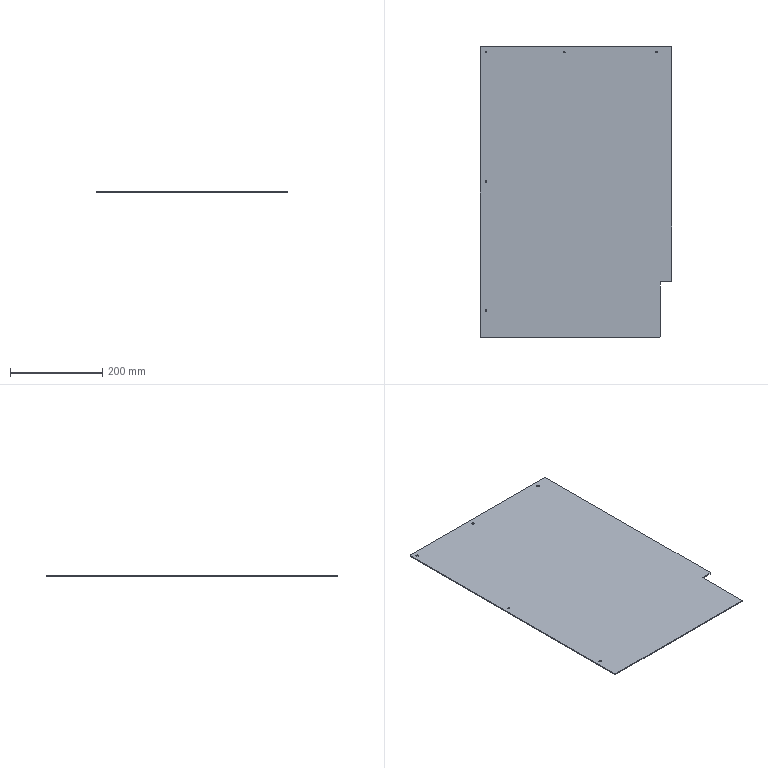Part | STEP file | 11-FG-JX01911 | 1 solid | 34 faces | box 415 x 630 x 2 mm | volume 516605 mm3 | cylinder 16 | cone 10 | plane 8 | commonest cylinder face diameters 3.4 x10 4 x6
STEP:
#1=CARTESIAN_POINT('',(-193.8,-257.,1.66));
#2=VERTEX_POINT('',#1);
#3=CARTESIAN_POINT('',(-197.2,-257.,1.66));
#4=VERTEX_POINT('',#3);
#5=CARTESIAN_POINT('',(-195.5,-257.,1.66));
#6=DIRECTION('',(0.,0.,-1.));
#7=DIRECTION('',(-1.,0.,0.));
#8=AXIS2_PLACEMENT_3D('',#5,#6,#7);
#9=CIRCLE('',#8,1.7);
#10=EDGE_CURVE('',#2,#4,#9,.T.);
#11=ORIENTED_EDGE('',*,*,#10,.F.);
#12=CARTESIAN_POINT('',(-192.14,-257.,0.));
#13=VERTEX_POINT('',#12);
#14=CARTESIAN_POINT('',(-192.14,-257.,0.));
#15=DIRECTION('',(0.7071,0.,-0.7071));
#16=VECTOR('',#15,1000.);
#17=LINE('',#14,#16);
#18=EDGE_CURVE('',#2,#13,#17,.T.);
#19=ORIENTED_EDGE('',*,*,#18,.T.);
#20=CARTESIAN_POINT('',(-198.86,-257.,0.));
#21=VERTEX_POINT('',#20);
#22=CARTESIAN_POINT('',(-195.5,-257.,0.));
#23=DIRECTION('',(0.,0.,-1.));
#24=DIRECTION('',(-1.,0.,0.));
#25=AXIS2_PLACEMENT_3D('',#22,#23,#24);
#26=CIRCLE('',#25,3.36);
#27=EDGE_CURVE('',#13,#21,#26,.T.);
#28=ORIENTED_EDGE('',*,*,#27,.T.);
#29=CARTESIAN_POINT('',(-198.86,-257.,0.));
#30=DIRECTION('',(-0.7071,0.,-0.7071));
#31=VECTOR('',#30,1000.);
#32=LINE('',#29,#31);
#33=EDGE_CURVE('',#4,#21,#32,.T.);
#34=ORIENTED_EDGE('',*,*,#33,.F.);
#35=EDGE_LOOP('',(#11,#19,#28,#34));
#36=FACE_OUTER_BOUND('',#35,.T.);
#37=CARTESIAN_POINT('',(-195.5,-257.,0.));
#38=DIRECTION('',(0.,0.,-1.));
#39=DIRECTION('',(-1.,0.,0.));
#40=AXIS2_PLACEMENT_3D('',#37,#38,#39);
#41=CONICAL_SURFACE('',#40,3.36,0.7854);
#42=ADVANCED_FACE('',(#36),#41,.F.);
#43=CARTESIAN_POINT('',(-193.8,-257.,2.));
#44=VERTEX_POINT('',#43);
#45=CARTESIAN_POINT('',(-197.2,-257.,2.));
#46=VERTEX_POINT('',#45);
#47=CARTESIAN_POINT('',(-195.5,-257.,2.));
#48=DIRECTION('',(0.,0.,-1.));
#49=DIRECTION('',(-1.,0.,0.));
#50=AXIS2_PLACEMENT_3D('',#47,#48,#49);
#51=CIRCLE('',#50,1.7);
#52=EDGE_CURVE('',#44,#46,#51,.T.);
#53=ORIENTED_EDGE('',*,*,#52,.F.);
#54=CARTESIAN_POINT('',(-193.8,-257.,0.));
#55=DIRECTION('',(0.,0.,-1.));
#56=VECTOR('',#55,1000.);
#57=LINE('',#54,#56);
#58=EDGE_CURVE('',#44,#2,#57,.T.);
#59=ORIENTED_EDGE('',*,*,#58,.T.);
#60=ORIENTED_EDGE('',*,*,#10,.T.);
#61=CARTESIAN_POINT('',(-197.2,-257.,0.));
#62=DIRECTION('',(0.,0.,-1.));
#63=VECTOR('',#62,1000.);
#64=LINE('',#61,#63);
#65=EDGE_CURVE('',#46,#4,#64,.T.);
#66=ORIENTED_EDGE('',*,*,#65,.F.);
#67=EDGE_LOOP('',(#53,#59,#60,#66));
#68=FACE_OUTER_BOUND('',#67,.T.);
#69=CARTESIAN_POINT('',(-195.5,-257.,0.));
#70=DIRECTION('',(0.,0.,-1.));
#71=DIRECTION('',(-1.,0.,0.));
#72=AXIS2_PLACEMENT_3D('',#69,#70,#71);
#73=CYLINDRICAL_SURFACE('',#72,1.7);
#74=ADVANCED_FACE('',(#68),#73,.F.);
#75=CARTESIAN_POINT('',(-193.8,23.,1.66));
#76=VERTEX_POINT('',#75);
#77=CARTESIAN_POINT('',(-197.2,23.,1.66));
#78=VERTEX_POINT('',#77);
#79=CARTESIAN_POINT('',(-195.5,23.,1.66));
#80=DIRECTION('',(0.,0.,-1.));
#81=DIRECTION('',(-1.,0.,0.));
#82=AXIS2_PLACEMENT_3D('',#79,#80,#81);
#83=CIRCLE('',#82,1.7);
#84=EDGE_CURVE('',#76,#78,#83,.T.);
#85=ORIENTED_EDGE('',*,*,#84,.F.);
#86=CARTESIAN_POINT('',(-192.14,23.,0.));
#87=VERTEX_POINT('',#86);
#88=CARTESIAN_POINT('',(-192.14,23.,0.));
#89=DIRECTION('',(0.7071,0.,-0.7071));
#90=VECTOR('',#89,1000.);
#91=LINE('',#88,#90);
#92=EDGE_CURVE('',#76,#87,#91,.T.);
#93=ORIENTED_EDGE('',*,*,#92,.T.);
#94=CARTESIAN_POINT('',(-198.86,23.,0.));
#95=VERTEX_POINT('',#94);
#96=CARTESIAN_POINT('',(-195.5,23.,0.));
#97=DIRECTION('',(0.,0.,-1.));
#98=DIRECTION('',(-1.,0.,0.));
#99=AXIS2_PLACEMENT_3D('',#96,#97,#98);
#100=CIRCLE('',#99,3.36);
#101=EDGE_CURVE('',#87,#95,#100,.T.);
#102=ORIENTED_EDGE('',*,*,#101,.T.);
#103=CARTESIAN_POINT('',(-198.86,23.,0.));
#104=DIRECTION('',(-0.7071,0.,-0.7071));
#105=VECTOR('',#104,1000.);
#106=LINE('',#103,#105);
#107=EDGE_CURVE('',#78,#95,#106,.T.);
#108=ORIENTED_EDGE('',*,*,#107,.F.);
#109=EDGE_LOOP('',(#85,#93,#102,#108));
#110=FACE_OUTER_BOUND('',#109,.T.);
#111=CARTESIAN_POINT('',(-195.5,23.,0.));
#112=DIRECTION('',(0.,0.,-1.));
#113=DIRECTION('',(-1.,0.,0.));
#114=AXIS2_PLACEMENT_3D('',#111,#112,#113);
#115=CONICAL_SURFACE('',#114,3.36,0.7854);
#116=ADVANCED_FACE('',(#110),#115,.F.);
#117=CARTESIAN_POINT('',(-193.8,23.,2.));
#118=VERTEX_POINT('',#117);
#119=CARTESIAN_POINT('',(-197.2,23.,2.));
#120=VERTEX_POINT('',#119);
#121=CARTESIAN_POINT('',(-195.5,23.,2.));
#122=DIRECTION('',(0.,0.,-1.));
#123=DIRECTION('',(-1.,0.,0.));
#124=AXIS2_PLACEMENT_3D('',#121,#122,#123);
#125=CIRCLE('',#124,1.7);
#126=EDGE_CURVE('',#118,#120,#125,.T.);
#127=ORIENTED_EDGE('',*,*,#126,.F.);
#128=CARTESIAN_POINT('',(-193.8,23.,0.));
#129=DIRECTION('',(0.,0.,-1.));
#130=VECTOR('',#129,1000.);
#131=LINE('',#128,#130);
#132=EDGE_CURVE('',#118,#76,#131,.T.);
#133=ORIENTED_EDGE('',*,*,#132,.T.);
#134=ORIENTED_EDGE('',*,*,#84,.T.);
#135=CARTESIAN_POINT('',(-197.2,23.,0.));
#136=DIRECTION('',(0.,0.,-1.));
#137=VECTOR('',#136,1000.);
#138=LINE('',#135,#137);
#139=EDGE_CURVE('',#120,#78,#138,.T.);
#140=ORIENTED_EDGE('',*,*,#139,.F.);
#141=EDGE_LOOP('',(#127,#133,#134,#140));
#142=FACE_OUTER_BOUND('',#141,.T.);
#143=CARTESIAN_POINT('',(-195.5,23.,0.));
#144=DIRECTION('',(0.,0.,-1.));
#145=DIRECTION('',(-1.,0.,0.));
#146=AXIS2_PLACEMENT_3D('',#143,#144,#145);
#147=CYLINDRICAL_SURFACE('',#146,1.7);
#148=ADVANCED_FACE('',(#142),#147,.F.);
#149=CARTESIAN_POINT('',(-193.8,303.,1.66));
#150=VERTEX_POINT('',#149);
#151=CARTESIAN_POINT('',(-197.2,303.,1.66));
#152=VERTEX_POINT('',#151);
#153=CARTESIAN_POINT('',(-195.5,303.,1.66));
#154=DIRECTION('',(0.,0.,-1.));
#155=DIRECTION('',(-1.,0.,0.));
#156=AXIS2_PLACEMENT_3D('',#153,#154,#155);
#157=CIRCLE('',#156,1.7);
#158=EDGE_CURVE('',#150,#152,#157,.T.);
#159=ORIENTED_EDGE('',*,*,#158,.F.);
#160=CARTESIAN_POINT('',(-192.14,303.,0.));
#161=VERTEX_POINT('',#160);
#162=CARTESIAN_POINT('',(-192.14,303.,0.));
#163=DIRECTION('',(0.7071,0.,-0.7071));
#164=VECTOR('',#163,1000.);
#165=LINE('',#162,#164);
#166=EDGE_CURVE('',#150,#161,#165,.T.);
#167=ORIENTED_EDGE('',*,*,#166,.T.);
#168=CARTESIAN_POINT('',(-198.86,303.,0.));
#169=VERTEX_POINT('',#168);
#170=CARTESIAN_POINT('',(-195.5,303.,0.));
#171=DIRECTION('',(0.,0.,-1.));
#172=DIRECTION('',(-1.,0.,0.));
#173=AXIS2_PLACEMENT_3D('',#170,#171,#172);
#174=CIRCLE('',#173,3.36);
#175=EDGE_CURVE('',#161,#169,#174,.T.);
#176=ORIENTED_EDGE('',*,*,#175,.T.);
#177=CARTESIAN_POINT('',(-198.86,303.,0.));
#178=DIRECTION('',(-0.7071,0.,-0.7071));
#179=VECTOR('',#178,1000.);
#180=LINE('',#177,#179);
#181=EDGE_CURVE('',#152,#169,#180,.T.);
#182=ORIENTED_EDGE('',*,*,#181,.F.);
#183=EDGE_LOOP('',(#159,#167,#176,#182));
#184=FACE_OUTER_BOUND('',#183,.T.);
#185=CARTESIAN_POINT('',(-195.5,303.,0.));
#186=DIRECTION('',(0.,0.,-1.));
#187=DIRECTION('',(-1.,0.,0.));
#188=AXIS2_PLACEMENT_3D('',#185,#186,#187);
#189=CONICAL_SURFACE('',#188,3.36,0.7854);
#190=ADVANCED_FACE('',(#184),#189,.F.);
#191=CARTESIAN_POINT('',(-193.8,303.,2.));
#192=VERTEX_POINT('',#191);
#193=CARTESIAN_POINT('',(-197.2,303.,2.));
#194=VERTEX_POINT('',#193);
#195=CARTESIAN_POINT('',(-195.5,303.,2.));
#196=DIRECTION('',(0.,0.,-1.));
#197=DIRECTION('',(-1.,0.,0.));
#198=AXIS2_PLACEMENT_3D('',#195,#196,#197);
#199=CIRCLE('',#198,1.7);
#200=EDGE_CURVE('',#192,#194,#199,.T.);
#201=ORIENTED_EDGE('',*,*,#200,.F.);
#202=CARTESIAN_POINT('',(-193.8,303.,0.));
#203=DIRECTION('',(0.,0.,-1.));
#204=VECTOR('',#203,1000.);
#205=LINE('',#202,#204);
#206=EDGE_CURVE('',#192,#150,#205,.T.);
#207=ORIENTED_EDGE('',*,*,#206,.T.);
#208=ORIENTED_EDGE('',*,*,#158,.T.);
#209=CARTESIAN_POINT('',(-197.2,303.,0.));
#210=DIRECTION('',(0.,0.,-1.));
#211=VECTOR('',#210,1000.);
#212=LINE('',#209,#211);
#213=EDGE_CURVE('',#194,#152,#212,.T.);
#214=ORIENTED_EDGE('',*,*,#213,.F.);
#215=EDGE_LOOP('',(#201,#207,#208,#214));
#216=FACE_OUTER_BOUND('',#215,.T.);
#217=CARTESIAN_POINT('',(-195.5,303.,0.));
#218=DIRECTION('',(0.,0.,-1.));
#219=DIRECTION('',(-1.,0.,0.));
#220=AXIS2_PLACEMENT_3D('',#217,#218,#219);
#221=CYLINDRICAL_SURFACE('',#220,1.7);
#222=ADVANCED_FACE('',(#216),#221,.F.);
#223=CARTESIAN_POINT('',(-23.8,303.,1.66));
#224=VERTEX_POINT('',#223);
#225=CARTESIAN_POINT('',(-27.2,303.,1.66));
#226=VERTEX_POINT('',#225);
#227=CARTESIAN_POINT('',(-25.5,303.,1.66));
#228=DIRECTION('',(0.,0.,-1.));
#229=DIRECTION('',(-1.,0.,0.));
#230=AXIS2_PLACEMENT_3D('',#227,#228,#229);
#231=CIRCLE('',#230,1.7);
#232=EDGE_CURVE('',#224,#226,#231,.T.);
#233=ORIENTED_EDGE('',*,*,#232,.F.);
#234=CARTESIAN_POINT('',(-22.14,303.,0.));
#235=VERTEX_POINT('',#234);
#236=CARTESIAN_POINT('',(-22.14,303.,0.));
#237=DIRECTION('',(0.7071,0.,-0.7071));
#238=VECTOR('',#237,1000.);
#239=LINE('',#236,#238);
#240=EDGE_CURVE('',#224,#235,#239,.T.);
#241=ORIENTED_EDGE('',*,*,#240,.T.);
#242=CARTESIAN_POINT('',(-28.86,303.,0.));
#243=VERTEX_POINT('',#242);
#244=CARTESIAN_POINT('',(-25.5,303.,0.));
#245=DIRECTION('',(0.,0.,-1.));
#246=DIRECTION('',(-1.,0.,0.));
#247=AXIS2_PLACEMENT_3D('',#244,#245,#246);
#248=CIRCLE('',#247,3.36);
#249=EDGE_CURVE('',#235,#243,#248,.T.);
#250=ORIENTED_EDGE('',*,*,#249,.T.);
#251=CARTESIAN_POINT('',(-28.86,303.,0.));
#252=DIRECTION('',(-0.7071,0.,-0.7071));
#253=VECTOR('',#252,1000.);
#254=LINE('',#251,#253);
#255=EDGE_CURVE('',#226,#243,#254,.T.);
#256=ORIENTED_EDGE('',*,*,#255,.F.);
#257=EDGE_LOOP('',(#233,#241,#250,#256));
#258=FACE_OUTER_BOUND('',#257,.T.);
#259=CARTESIAN_POINT('',(-25.5,303.,0.));
#260=DIRECTION('',(0.,0.,-1.));
#261=DIRECTION('',(-1.,0.,0.));
#262=AXIS2_PLACEMENT_3D('',#259,#260,#261);
#263=CONICAL_SURFACE('',#262,3.36,0.7854);
#264=ADVANCED_FACE('',(#258),#263,.F.);
#265=CARTESIAN_POINT('',(-23.8,303.,2.));
#266=VERTEX_POINT('',#265);
#267=CARTESIAN_POINT('',(-27.2,303.,2.));
#268=VERTEX_POINT('',#267);
#269=CARTESIAN_POINT('',(-25.5,303.,2.));
#270=DIRECTION('',(0.,0.,-1.));
#271=DIRECTION('',(-1.,0.,0.));
#272=AXIS2_PLACEMENT_3D('',#269,#270,#271);
#273=CIRCLE('',#272,1.7);
#274=EDGE_CURVE('',#266,#268,#273,.T.);
#275=ORIENTED_EDGE('',*,*,#274,.F.);
#276=CARTESIAN_POINT('',(-23.8,303.,0.));
#277=DIRECTION('',(0.,0.,-1.));
#278=VECTOR('',#277,1000.);
#279=LINE('',#276,#278);
#280=EDGE_CURVE('',#266,#224,#279,.T.);
#281=ORIENTED_EDGE('',*,*,#280,.T.);
#282=ORIENTED_EDGE('',*,*,#232,.T.);
#283=CARTESIAN_POINT('',(-27.2,303.,0.));
#284=DIRECTION('',(0.,0.,-1.));
#285=VECTOR('',#284,1000.);
#286=LINE('',#283,#285);
#287=EDGE_CURVE('',#268,#226,#286,.T.);
#288=ORIENTED_EDGE('',*,*,#287,.F.);
#289=EDGE_LOOP('',(#275,#281,#282,#288));
#290=FACE_OUTER_BOUND('',#289,.T.);
#291=CARTESIAN_POINT('',(-25.5,303.,0.));
#292=DIRECTION('',(0.,0.,-1.));
#293=DIRECTION('',(-1.,0.,0.));
#294=AXIS2_PLACEMENT_3D('',#291,#292,#293);
#295=CYLINDRICAL_SURFACE('',#294,1.7);
#296=ADVANCED_FACE('',(#290),#295,.F.);
#297=CARTESIAN_POINT('',(176.2,303.,1.66));
#298=VERTEX_POINT('',#297);
#299=CARTESIAN_POINT('',(172.8,303.,1.66));
#300=VERTEX_POINT('',#299);
#301=CARTESIAN_POINT('',(174.5,303.,1.66));
#302=DIRECTION('',(0.,0.,-1.));
#303=DIRECTION('',(-1.,0.,0.));
#304=AXIS2_PLACEMENT_3D('',#301,#302,#303);
#305=CIRCLE('',#304,1.7);
#306=EDGE_CURVE('',#298,#300,#305,.T.);
#307=ORIENTED_EDGE('',*,*,#306,.F.);
#308=CARTESIAN_POINT('',(177.86,303.,0.));
#309=VERTEX_POINT('',#308);
#310=CARTESIAN_POINT('',(177.86,303.,0.));
#311=DIRECTION('',(0.7071,0.,-0.7071));
#312=VECTOR('',#311,1000.);
#313=LINE('',#310,#312);
#314=EDGE_CURVE('',#298,#309,#313,.T.);
#315=ORIENTED_EDGE('',*,*,#314,.T.);
#316=CARTESIAN_POINT('',(171.14,303.,0.));
#317=VERTEX_POINT('',#316);
#318=CARTESIAN_POINT('',(174.5,303.,0.));
#319=DIRECTION('',(0.,0.,-1.));
#320=DIRECTION('',(-1.,0.,0.));
#321=AXIS2_PLACEMENT_3D('',#318,#319,#320);
#322=CIRCLE('',#321,3.36);
#323=EDGE_CURVE('',#309,#317,#322,.T.);
#324=ORIENTED_EDGE('',*,*,#323,.T.);
#325=CARTESIAN_POINT('',(171.14,303.,0.));
#326=DIRECTION('',(-0.7071,0.,-0.7071));
#327=VECTOR('',#326,1000.);
#328=LINE('',#325,#327);
#329=EDGE_CURVE('',#300,#317,#328,.T.);
#330=ORIENTED_EDGE('',*,*,#329,.F.);
#331=EDGE_LOOP('',(#307,#315,#324,#330));
#332=FACE_OUTER_BOUND('',#331,.T.);
#333=CARTESIAN_POINT('',(174.5,303.,0.));
#334=DIRECTION('',(0.,0.,-1.));
#335=DIRECTION('',(-1.,0.,0.));
#336=AXIS2_PLACEMENT_3D('',#333,#334,#335);
#337=CONICAL_SURFACE('',#336,3.36,0.7854);
#338=ADVANCED_FACE('',(#332),#337,.F.);
#339=CARTESIAN_POINT('',(176.2,303.,2.));
#340=VERTEX_POINT('',#339);
#341=CARTESIAN_POINT('',(172.8,303.,2.));
#342=VERTEX_POINT('',#341);
#343=CARTESIAN_POINT('',(174.5,303.,2.));
#344=DIRECTION('',(0.,0.,-1.));
#345=DIRECTION('',(-1.,0.,0.));
#346=AXIS2_PLACEMENT_3D('',#343,#344,#345);
#347=CIRCLE('',#346,1.7);
#348=EDGE_CURVE('',#340,#342,#347,.T.);
#349=ORIENTED_EDGE('',*,*,#348,.F.);
#350=CARTESIAN_POINT('',(176.2,303.,0.));
#351=DIRECTION('',(0.,0.,-1.));
#352=VECTOR('',#351,1000.);
#353=LINE('',#350,#352);
#354=EDGE_CURVE('',#340,#298,#353,.T.);
#355=ORIENTED_EDGE('',*,*,#354,.T.);
#356=ORIENTED_EDGE('',*,*,#306,.T.);
#357=CARTESIAN_POINT('',(172.8,303.,0.));
#358=DIRECTION('',(0.,0.,-1.));
#359=VECTOR('',#358,1000.);
#360=LINE('',#357,#359);
#361=EDGE_CURVE('',#342,#300,#360,.T.);
#362=ORIENTED_EDGE('',*,*,#361,.F.);
#363=EDGE_LOOP('',(#349,#355,#356,#362));
#364=FACE_OUTER_BOUND('',#363,.T.);
#365=CARTESIAN_POINT('',(174.5,303.,0.));
#366=DIRECTION('',(0.,0.,-1.));
#367=DIRECTION('',(-1.,0.,0.));
#368=AXIS2_PLACEMENT_3D('',#365,#366,#367);
#369=CYLINDRICAL_SURFACE('',#368,1.7);
#370=ADVANCED_FACE('',(#364),#369,.F.);
#371=CARTESIAN_POINT('',(207.5,-191.,2.));
#372=VERTEX_POINT('',#371);
#373=CARTESIAN_POINT('',(207.5,313.,2.));
#374=VERTEX_POINT('',#373);
#375=CARTESIAN_POINT('',(207.5,315.,2.));
#376=DIRECTION('',(0.,1.,0.));
#377=VECTOR('',#376,1000.);
#378=LINE('',#375,#377);
#379=EDGE_CURVE('',#372,#374,#378,.T.);
#380=ORIENTED_EDGE('',*,*,#379,.F.);
#381=CARTESIAN_POINT('',(207.5,-191.,0.));
#382=VERTEX_POINT('',#381);
#383=CARTESIAN_POINT('',(207.5,-191.,2.));
#384=DIRECTION('',(0.,0.,-1.));
#385=VECTOR('',#384,1000.);
#386=LINE('',#383,#385);
#387=EDGE_CURVE('',#372,#382,#386,.T.);
#388=ORIENTED_EDGE('',*,*,#387,.T.);
#389=CARTESIAN_POINT('',(207.5,313.,0.));
#390=VERTEX_POINT('',#389);
#391=CARTESIAN_POINT('',(207.5,315.,0.));
#392=DIRECTION('',(0.,1.,0.));
#393=VECTOR('',#392,1000.);
#394=LINE('',#391,#393);
#395=EDGE_CURVE('',#382,#390,#394,.T.);
#396=ORIENTED_EDGE('',*,*,#395,.T.);
#397=CARTESIAN_POINT('',(207.5,313.,2.));
#398=DIRECTION('',(0.,0.,1.));
#399=VECTOR('',#398,1000.);
#400=LINE('',#397,#399);
#401=EDGE_CURVE('',#390,#374,#400,.T.);
#402=ORIENTED_EDGE('',*,*,#401,.T.);
#403=EDGE_LOOP('',(#380,#388,#396,#402));
#404=FACE_OUTER_BOUND('',#403,.T.);
#405=CARTESIAN_POINT('',(207.5,315.,2.));
#406=DIRECTION('',(-1.,0.,0.));
#407=DIRECTION('',(0.,-1.,0.));
#408=AXIS2_PLACEMENT_3D('',#405,#406,#407);
#409=PLANE('',#408);
#410=ADVANCED_FACE('',(#404),#409,.F.);
#411=CARTESIAN_POINT('',(205.5,315.,2.));
#412=VERTEX_POINT('',#411);
#413=CARTESIAN_POINT('',(-205.5,315.,2.));
#414=VERTEX_POINT('',#413);
#415=CARTESIAN_POINT('',(-207.5,315.,2.));
#416=DIRECTION('',(-1.,0.,0.));
#417=VECTOR('',#416,1000.);
#418=LINE('',#415,#417);
#419=EDGE_CURVE('',#412,#414,#418,.T.);
#420=ORIENTED_EDGE('',*,*,#419,.F.);
#421=CARTESIAN_POINT('',(205.5,315.,0.));
#422=VERTEX_POINT('',#421);
#423=CARTESIAN_POINT('',(205.5,315.,2.));
#424=DIRECTION('',(0.,0.,-1.));
#425=VECTOR('',#424,1000.);
#426=LINE('',#423,#425);
#427=EDGE_CURVE('',#412,#422,#426,.T.);
#428=ORIENTED_EDGE('',*,*,#427,.T.);
#429=CARTESIAN_POINT('',(-205.5,315.,0.));
#430=VERTEX_POINT('',#429);
#431=CARTESIAN_POINT('',(-207.5,315.,0.));
#432=DIRECTION('',(-1.,0.,0.));
#433=VECTOR('',#432,1000.);
#434=LINE('',#431,#433);
#435=EDGE_CURVE('',#422,#430,#434,.T.);
#436=ORIENTED_EDGE('',*,*,#435,.T.);
#437=CARTESIAN_POINT('',(-205.5,315.,2.));
#438=DIRECTION('',(0.,0.,1.));
#439=VECTOR('',#438,1000.);
#440=LINE('',#437,#439);
#441=EDGE_CURVE('',#430,#414,#440,.T.);
#442=ORIENTED_EDGE('',*,*,#441,.T.);
#443=EDGE_LOOP('',(#420,#428,#436,#442));
#444=FACE_OUTER_BOUND('',#443,.T.);
#445=CARTESIAN_POINT('',(-207.5,315.,2.));
#446=DIRECTION('',(0.,-1.,0.));
#447=DIRECTION('',(0.,0.,-1.));
#448=AXIS2_PLACEMENT_3D('',#445,#446,#447);
#449=PLANE('',#448);
#450=ADVANCED_FACE('',(#444),#449,.F.);
#451=CARTESIAN_POINT('',(-207.5,313.,0.));
#452=VERTEX_POINT('',#451);
#453=CARTESIAN_POINT('',(-207.5,-313.,0.));
#454=VERTEX_POINT('',#453);
#455=CARTESIAN_POINT('',(-207.5,315.,0.));
#456=DIRECTION('',(0.,-1.,0.));
#457=VECTOR('',#456,1000.);
#458=LINE('',#455,#457);
#459=EDGE_CURVE('',#452,#454,#458,.T.);
#460=ORIENTED_EDGE('',*,*,#459,.T.);
#461=CARTESIAN_POINT('',(-207.5,-313.,2.));
#462=VERTEX_POINT('',#461);
#463=CARTESIAN_POINT('',(-207.5,-313.,2.));
#464=DIRECTION('',(0.,0.,1.));
#465=VECTOR('',#464,1000.);
#466=LINE('',#463,#465);
#467=EDGE_CURVE('',#454,#462,#466,.T.);
#468=ORIENTED_EDGE('',*,*,#467,.T.);
#469=CARTESIAN_POINT('',(-207.5,313.,2.));
#470=VERTEX_POINT('',#469);
#471=CARTESIAN_POINT('',(-207.5,315.,2.));
#472=DIRECTION('',(0.,-1.,0.));
#473=VECTOR('',#472,1000.);
#474=LINE('',#471,#473);
#475=EDGE_CURVE('',#470,#462,#474,.T.);
#476=ORIENTED_EDGE('',*,*,#475,.F.);
#477=CARTESIAN_POINT('',(-207.5,313.,2.));
#478=DIRECTION('',(0.,0.,-1.));
#479=VECTOR('',#478,1000.);
#480=LINE('',#477,#479);
#481=EDGE_CURVE('',#470,#452,#480,.T.);
#482=ORIENTED_EDGE('',*,*,#481,.T.);
#483=EDGE_LOOP('',(#460,#468,#476,#482));
#484=FACE_OUTER_BOUND('',#483,.T.);
#485=CARTESIAN_POINT('',(-207.5,315.,2.));
#486=DIRECTION('',(1.,0.,0.));
#487=DIRECTION('',(0.,1.,0.));
#488=AXIS2_PLACEMENT_3D('',#485,#486,#487);
#489=PLANE('',#488);
#490=ADVANCED_FACE('',(#484),#489,.F.);
#491=CARTESIAN_POINT('',(-205.5,-315.,2.));
#492=VERTEX_POINT('',#491);
#493=CARTESIAN_POINT('',(180.5,-315.,2.));
#494=VERTEX_POINT('',#493);
#495=CARTESIAN_POINT('',(-207.5,-315.,2.));
#496=DIRECTION('',(1.,0.,0.));
#497=VECTOR('',#496,1000.);
#498=LINE('',#495,#497);
#499=EDGE_CURVE('',#492,#494,#498,.T.);
#500=ORIENTED_EDGE('',*,*,#499,.F.);
#501=CARTESIAN_POINT('',(-205.5,-315.,0.));
#502=VERTEX_POINT('',#501);
#503=CARTESIAN_POINT('',(-205.5,-315.,2.));
#504=DIRECTION('',(0.,0.,-1.));
#505=VECTOR('',#504,1000.);
#506=LINE('',#503,#505);
#507=EDGE_CURVE('',#492,#502,#506,.T.);
#508=ORIENTED_EDGE('',*,*,#507,.T.);
#509=CARTESIAN_POINT('',(180.5,-315.,0.));
#510=VERTEX_POINT('',#509);
#511=CARTESIAN_POINT('',(-207.5,-315.,0.));
#512=DIRECTION('',(1.,0.,0.));
#513=VECTOR('',#512,1000.);
#514=LINE('',#511,#513);
#515=EDGE_CURVE('',#502,#510,#514,.T.);
#516=ORIENTED_EDGE('',*,*,#515,.T.);
#517=CARTESIAN_POINT('',(180.5,-315.,2.));
#518=DIRECTION('',(0.,0.,1.));
#519=VECTOR('',#518,1000.);
#520=LINE('',#517,#519);
#521=EDGE_CURVE('',#510,#494,#520,.T.);
#522=ORIENTED_EDGE('',*,*,#521,.T.);
#523=EDGE_LOOP('',(#500,#508,#516,#522));
#524=FACE_OUTER_BOUND('',#523,.T.);
#525=CARTESIAN_POINT('',(-207.5,-315.,2.));
#526=DIRECTION('',(0.,1.,0.));
#527=DIRECTION('',(0.,0.,1.));
#528=AXIS2_PLACEMENT_3D('',#525,#526,#527);
#529=PLANE('',#528);
#530=ADVANCED_FACE('',(#524),#529,.F.);
#531=CARTESIAN_POINT('',(-195.5,-257.,2.));
#532=DIRECTION('',(0.,0.,-1.));
#533=DIRECTION('',(-1.,0.,0.));
#534=AXIS2_PLACEMENT_3D('',#531,#532,#533);
#535=CIRCLE('',#534,1.7);
#536=EDGE_CURVE('',#46,#44,#535,.T.);
#537=ORIENTED_EDGE('',*,*,#536,.T.);
#538=ORIENTED_EDGE('',*,*,#52,.T.);
#539=EDGE_LOOP('',(#537,#538));
#540=FACE_BOUND('',#539,.T.);
#541=CARTESIAN_POINT('',(-195.5,23.,2.));
#542=DIRECTION('',(0.,0.,-1.));
#543=DIRECTION('',(-1.,0.,0.));
#544=AXIS2_PLACEMENT_3D('',#541,#542,#543);
#545=CIRCLE('',#544,1.7);
#546=EDGE_CURVE('',#120,#118,#545,.T.);
#547=ORIENTED_EDGE('',*,*,#546,.T.);
#548=ORIENTED_EDGE('',*,*,#126,.T.);
#549=EDGE_LOOP('',(#547,#548));
#550=FACE_BOUND('',#549,.T.);
#551=CARTESIAN_POINT('',(-195.5,303.,2.));
#552=DIRECTION('',(0.,0.,-1.));
#553=DIRECTION('',(-1.,0.,0.));
#554=AXIS2_PLACEMENT_3D('',#551,#552,#553);
#555=CIRCLE('',#554,1.7);
#556=EDGE_CURVE('',#194,#192,#555,.T.);
#557=ORIENTED_EDGE('',*,*,#556,.T.);
#558=ORIENTED_EDGE('',*,*,#200,.T.);
#559=EDGE_LOOP('',(#557,#558));
#560=FACE_BOUND('',#559,.T.);
#561=CARTESIAN_POINT('',(-25.5,303.,2.));
#562=DIRECTION('',(0.,0.,-1.));
#563=DIRECTION('',(-1.,0.,0.));
#564=AXIS2_PLACEMENT_3D('',#561,#562,#563);
#565=CIRCLE('',#564,1.7);
#566=EDGE_CURVE('',#268,#266,#565,.T.);
#567=ORIENTED_EDGE('',*,*,#566,.T.);
#568=ORIENTED_EDGE('',*,*,#274,.T.);
#569=EDGE_LOOP('',(#567,#568));
#570=FACE_BOUND('',#569,.T.);
#571=CARTESIAN_POINT('',(174.5,303.,2.));
#572=DIRECTION('',(0.,0.,-1.));
#573=DIRECTION('',(-1.,0.,0.));
#574=AXIS2_PLACEMENT_3D('',#571,#572,#573);
#575=CIRCLE('',#574,1.7);
#576=EDGE_CURVE('',#342,#340,#575,.T.);
#577=ORIENTED_EDGE('',*,*,#576,.T.);
#578=ORIENTED_EDGE('',*,*,#348,.T.);
#579=EDGE_LOOP('',(#577,#578));
#580=FACE_BOUND('',#579,.T.);
#581=ORIENTED_EDGE('',*,*,#475,.T.);
#582=CARTESIAN_POINT('',(-205.5,-313.,2.));
#583=DIRECTION('',(0.,0.,1.));
#584=DIRECTION('',(1.,0.,0.));
#585=AXIS2_PLACEMENT_3D('',#582,#583,#584);
#586=CIRCLE('',#585,2.);
#587=EDGE_CURVE('',#462,#492,#586,.T.);
#588=ORIENTED_EDGE('',*,*,#587,.T.);
#589=ORIENTED_EDGE('',*,*,#499,.T.);
#590=CARTESIAN_POINT('',(182.5,-313.,2.));
#591=VERTEX_POINT('',#590);
#592=CARTESIAN_POINT('',(180.5,-313.,2.));
#593=DIRECTION('',(0.,0.,1.));
#594=DIRECTION('',(1.,0.,0.));
#595=AXIS2_PLACEMENT_3D('',#592,#593,#594);
#596=CIRCLE('',#595,2.);
#597=EDGE_CURVE('',#494,#591,#596,.T.);
#598=ORIENTED_EDGE('',*,*,#597,.T.);
#599=CARTESIAN_POINT('',(182.5,-195.,2.));
#600=VERTEX_POINT('',#599);
#601=CARTESIAN_POINT('',(182.5,0.,2.));
#602=DIRECTION('',(0.,-1.,0.));
#603=VECTOR('',#602,1000.);
#604=LINE('',#601,#603);
#605=EDGE_CURVE('',#600,#591,#604,.T.);
#606=ORIENTED_EDGE('',*,*,#605,.F.);
#607=CARTESIAN_POINT('',(184.5,-193.,2.));
#608=VERTEX_POINT('',#607);
#609=CARTESIAN_POINT('',(184.5,-195.,2.));
#610=DIRECTION('',(0.,0.,-1.));
#611=DIRECTION('',(1.,0.,0.));
#612=AXIS2_PLACEMENT_3D('',#609,#610,#611);
#613=CIRCLE('',#612,2.);
#614=EDGE_CURVE('',#600,#608,#613,.T.);
#615=ORIENTED_EDGE('',*,*,#614,.T.);
#616=CARTESIAN_POINT('',(205.5,-193.,2.));
#617=VERTEX_POINT('',#616);
#618=CARTESIAN_POINT('',(0.,-193.,2.));
#619=DIRECTION('',(-1.,0.,0.));
#620=VECTOR('',#619,1000.);
#621=LINE('',#618,#620);
#622=EDGE_CURVE('',#617,#608,#621,.T.);
#623=ORIENTED_EDGE('',*,*,#622,.F.);
#624=CARTESIAN_POINT('',(205.5,-191.,2.));
#625=DIRECTION('',(0.,0.,1.));
#626=DIRECTION('',(1.,0.,0.));
#627=AXIS2_PLACEMENT_3D('',#624,#625,#626);
#628=CIRCLE('',#627,2.);
#629=EDGE_CURVE('',#617,#372,#628,.T.);
#630=ORIENTED_EDGE('',*,*,#629,.T.);
#631=ORIENTED_EDGE('',*,*,#379,.T.);
#632=CARTESIAN_POINT('',(205.5,313.,2.));
#633=DIRECTION('',(0.,0.,1.));
#634=DIRECTION('',(1.,0.,0.));
#635=AXIS2_PLACEMENT_3D('',#632,#633,#634);
#636=CIRCLE('',#635,2.);
#637=EDGE_CURVE('',#374,#412,#636,.T.);
#638=ORIENTED_EDGE('',*,*,#637,.T.);
#639=ORIENTED_EDGE('',*,*,#419,.T.);
#640=CARTESIAN_POINT('',(-205.5,313.,2.));
#641=DIRECTION('',(0.,0.,1.));
#642=DIRECTION('',(1.,0.,0.));
#643=AXIS2_PLACEMENT_3D('',#640,#641,#642);
#644=CIRCLE('',#643,2.);
#645=EDGE_CURVE('',#414,#470,#644,.T.);
#646=ORIENTED_EDGE('',*,*,#645,.T.);
#647=EDGE_LOOP('',(#581,#588,#589,#598,#606,#615,#623,#630,#631,#638,#639,#646));
#648=FACE_OUTER_BOUND('',#647,.T.);
#649=CARTESIAN_POINT('',(0.,0.,2.));
#650=DIRECTION('',(0.,0.,1.));
#651=DIRECTION('',(1.,0.,0.));
#652=AXIS2_PLACEMENT_3D('',#649,#650,#651);
#653=PLANE('',#652);
#654=ADVANCED_FACE('',(#540,#550,#560,#570,#580,#648),#653,.T.);
#655=CARTESIAN_POINT('',(-195.5,-257.,0.));
#656=DIRECTION('',(0.,0.,-1.));
#657=DIRECTION('',(-1.,0.,0.));
#658=AXIS2_PLACEMENT_3D('',#655,#656,#657);
#659=CIRCLE('',#658,3.36);
#660=EDGE_CURVE('',#21,#13,#659,.T.);
#661=ORIENTED_EDGE('',*,*,#660,.F.);
#662=ORIENTED_EDGE('',*,*,#27,.F.);
#663=EDGE_LOOP('',(#661,#662));
#664=FACE_BOUND('',#663,.T.);
#665=CARTESIAN_POINT('',(-195.5,23.,0.));
#666=DIRECTION('',(0.,0.,-1.));
#667=DIRECTION('',(-1.,0.,0.));
#668=AXIS2_PLACEMENT_3D('',#665,#666,#667);
#669=CIRCLE('',#668,3.36);
#670=EDGE_CURVE('',#95,#87,#669,.T.);
#671=ORIENTED_EDGE('',*,*,#670,.F.);
#672=ORIENTED_EDGE('',*,*,#101,.F.);
#673=EDGE_LOOP('',(#671,#672));
#674=FACE_BOUND('',#673,.T.);
#675=CARTESIAN_POINT('',(-195.5,303.,0.));
#676=DIRECTION('',(0.,0.,-1.));
#677=DIRECTION('',(-1.,0.,0.));
#678=AXIS2_PLACEMENT_3D('',#675,#676,#677);
#679=CIRCLE('',#678,3.36);
#680=EDGE_CURVE('',#169,#161,#679,.T.);
#681=ORIENTED_EDGE('',*,*,#680,.F.);
#682=ORIENTED_EDGE('',*,*,#175,.F.);
#683=EDGE_LOOP('',(#681,#682));
#684=FACE_BOUND('',#683,.T.);
#685=CARTESIAN_POINT('',(-25.5,303.,0.));
#686=DIRECTION('',(0.,0.,-1.));
#687=DIRECTION('',(-1.,0.,0.));
#688=AXIS2_PLACEMENT_3D('',#685,#686,#687);
#689=CIRCLE('',#688,3.36);
#690=EDGE_CURVE('',#243,#235,#689,.T.);
#691=ORIENTED_EDGE('',*,*,#690,.F.);
#692=ORIENTED_EDGE('',*,*,#249,.F.);
#693=EDGE_LOOP('',(#691,#692));
#694=FACE_BOUND('',#693,.T.);
#695=CARTESIAN_POINT('',(174.5,303.,0.));
#696=DIRECTION('',(0.,0.,-1.));
#697=DIRECTION('',(-1.,0.,0.));
#698=AXIS2_PLACEMENT_3D('',#695,#696,#697);
#699=CIRCLE('',#698,3.36);
#700=EDGE_CURVE('',#317,#309,#699,.T.);
#701=ORIENTED_EDGE('',*,*,#700,.F.);
#702=ORIENTED_EDGE('',*,*,#323,.F.);
#703=EDGE_LOOP('',(#701,#702));
#704=FACE_BOUND('',#703,.T.);
#705=ORIENTED_EDGE('',*,*,#515,.F.);
#706=CARTESIAN_POINT('',(-205.5,-313.,0.));
#707=DIRECTION('',(0.,0.,-1.));
#708=DIRECTION('',(1.,0.,0.));
#709=AXIS2_PLACEMENT_3D('',#706,#707,#708);
#710=CIRCLE('',#709,2.);
#711=EDGE_CURVE('',#502,#454,#710,.T.);
#712=ORIENTED_EDGE('',*,*,#711,.T.);
#713=ORIENTED_EDGE('',*,*,#459,.F.);
#714=CARTESIAN_POINT('',(-205.5,313.,0.));
#715=DIRECTION('',(0.,0.,-1.));
#716=DIRECTION('',(1.,0.,0.));
#717=AXIS2_PLACEMENT_3D('',#714,#715,#716);
#718=CIRCLE('',#717,2.);
#719=EDGE_CURVE('',#452,#430,#718,.T.);
#720=ORIENTED_EDGE('',*,*,#719,.T.);
#721=ORIENTED_EDGE('',*,*,#435,.F.);
#722=CARTESIAN_POINT('',(205.5,313.,0.));
#723=DIRECTION('',(0.,0.,-1.));
#724=DIRECTION('',(1.,0.,0.));
#725=AXIS2_PLACEMENT_3D('',#722,#723,#724);
#726=CIRCLE('',#725,2.);
#727=EDGE_CURVE('',#422,#390,#726,.T.);
#728=ORIENTED_EDGE('',*,*,#727,.T.);
#729=ORIENTED_EDGE('',*,*,#395,.F.);
#730=CARTESIAN_POINT('',(205.5,-193.,0.));
#731=VERTEX_POINT('',#730);
#732=CARTESIAN_POINT('',(205.5,-191.,0.));
#733=DIRECTION('',(0.,0.,-1.));
#734=DIRECTION('',(1.,0.,0.));
#735=AXIS2_PLACEMENT_3D('',#732,#733,#734);
#736=CIRCLE('',#735,2.);
#737=EDGE_CURVE('',#382,#731,#736,.T.);
#738=ORIENTED_EDGE('',*,*,#737,.T.);
#739=CARTESIAN_POINT('',(184.5,-193.,0.));
#740=VERTEX_POINT('',#739);
#741=CARTESIAN_POINT('',(207.5,-193.,0.));
#742=DIRECTION('',(1.,0.,0.));
#743=VECTOR('',#742,1000.);
#744=LINE('',#741,#743);
#745=EDGE_CURVE('',#740,#731,#744,.T.);
#746=ORIENTED_EDGE('',*,*,#745,.F.);
#747=CARTESIAN_POINT('',(182.5,-195.,0.));
#748=VERTEX_POINT('',#747);
#749=CARTESIAN_POINT('',(184.5,-195.,0.));
#750=DIRECTION('',(0.,0.,1.));
#751=DIRECTION('',(1.,0.,0.));
#752=AXIS2_PLACEMENT_3D('',#749,#750,#751);
#753=CIRCLE('',#752,2.);
#754=EDGE_CURVE('',#740,#748,#753,.T.);
#755=ORIENTED_EDGE('',*,*,#754,.T.);
#756=CARTESIAN_POINT('',(182.5,-313.,0.));
#757=VERTEX_POINT('',#756);
#758=CARTESIAN_POINT('',(182.5,-315.,0.));
#759=DIRECTION('',(0.,1.,0.));
#760=VECTOR('',#759,1000.);
#761=LINE('',#758,#760);
#762=EDGE_CURVE('',#757,#748,#761,.T.);
#763=ORIENTED_EDGE('',*,*,#762,.F.);
#764=CARTESIAN_POINT('',(180.5,-313.,0.));
#765=DIRECTION('',(0.,0.,-1.));
#766=DIRECTION('',(1.,0.,0.));
#767=AXIS2_PLACEMENT_3D('',#764,#765,#766);
#768=CIRCLE('',#767,2.);
#769=EDGE_CURVE('',#757,#510,#768,.T.);
#770=ORIENTED_EDGE('',*,*,#769,.T.);
#771=EDGE_LOOP('',(#705,#712,#713,#720,#721,#728,#729,#738,#746,#755,#763,#770));
#772=FACE_OUTER_BOUND('',#771,.T.);
#773=CARTESIAN_POINT('',(0.,0.,0.));
#774=DIRECTION('',(0.,0.,1.));
#775=DIRECTION('',(1.,0.,0.));
#776=AXIS2_PLACEMENT_3D('',#773,#774,#775);
#777=PLANE('',#776);
#778=ADVANCED_FACE('',(#664,#674,#684,#694,#704,#772),#777,.F.);
#779=ORIENTED_EDGE('',*,*,#745,.T.);
#780=CARTESIAN_POINT('',(205.5,-193.,10.));
#781=DIRECTION('',(0.,0.,1.));
#782=VECTOR('',#781,1000.);
#783=LINE('',#780,#782);
#784=EDGE_CURVE('',#731,#617,#783,.T.);
#785=ORIENTED_EDGE('',*,*,#784,.T.);
#786=ORIENTED_EDGE('',*,*,#622,.T.);
#787=CARTESIAN_POINT('',(184.5,-193.,0.));
#788=DIRECTION('',(0.,0.,-1.));
#789=VECTOR('',#788,1000.);
#790=LINE('',#787,#789);
#791=EDGE_CURVE('',#608,#740,#790,.T.);
#792=ORIENTED_EDGE('',*,*,#791,.T.);
#793=EDGE_LOOP('',(#779,#785,#786,#792));
#794=FACE_OUTER_BOUND('',#793,.T.);
#795=CARTESIAN_POINT('',(207.5,-193.,10.));
#796=DIRECTION('',(0.,1.,0.));
#797=DIRECTION('',(0.,0.,1.));
#798=AXIS2_PLACEMENT_3D('',#795,#796,#797);
#799=PLANE('',#798);
#800=ADVANCED_FACE('',(#794),#799,.F.);
#801=ORIENTED_EDGE('',*,*,#605,.T.);
#802=CARTESIAN_POINT('',(182.5,-313.,10.));
#803=DIRECTION('',(0.,0.,-1.));
#804=VECTOR('',#803,1000.);
#805=LINE('',#802,#804);
#806=EDGE_CURVE('',#591,#757,#805,.T.);
#807=ORIENTED_EDGE('',*,*,#806,.T.);
#808=ORIENTED_EDGE('',*,*,#762,.T.);
#809=CARTESIAN_POINT('',(182.5,-195.,2.));
#810=DIRECTION('',(0.,0.,1.));
#811=VECTOR('',#810,1000.);
#812=LINE('',#809,#811);
#813=EDGE_CURVE('',#748,#600,#812,.T.);
#814=ORIENTED_EDGE('',*,*,#813,.T.);
#815=EDGE_LOOP('',(#801,#807,#808,#814));
#816=FACE_OUTER_BOUND('',#815,.T.);
#817=CARTESIAN_POINT('',(182.5,-315.,10.));
#818=DIRECTION('',(-1.,0.,0.));
#819=DIRECTION('',(0.,0.,1.));
#820=AXIS2_PLACEMENT_3D('',#817,#818,#819);
#821=PLANE('',#820);
#822=ADVANCED_FACE('',(#816),#821,.F.);
#823=ORIENTED_EDGE('',*,*,#354,.F.);
#824=ORIENTED_EDGE('',*,*,#576,.F.);
#825=ORIENTED_EDGE('',*,*,#361,.T.);
#826=CARTESIAN_POINT('',(174.5,303.,1.66));
#827=DIRECTION('',(0.,0.,-1.));
#828=DIRECTION('',(-1.,0.,0.));
#829=AXIS2_PLACEMENT_3D('',#826,#827,#828);
#830=CIRCLE('',#829,1.7);
#831=EDGE_CURVE('',#300,#298,#830,.T.);
#832=ORIENTED_EDGE('',*,*,#831,.T.);
#833=EDGE_LOOP('',(#823,#824,#825,#832));
#834=FACE_OUTER_BOUND('',#833,.T.);
#835=CARTESIAN_POINT('',(174.5,303.,0.));
#836=DIRECTION('',(0.,0.,-1.));
#837=DIRECTION('',(-1.,0.,0.));
#838=AXIS2_PLACEMENT_3D('',#835,#836,#837);
#839=CYLINDRICAL_SURFACE('',#838,1.7);
#840=ADVANCED_FACE('',(#834),#839,.F.);
#841=ORIENTED_EDGE('',*,*,#314,.F.);
#842=ORIENTED_EDGE('',*,*,#831,.F.);
#843=ORIENTED_EDGE('',*,*,#329,.T.);
#844=ORIENTED_EDGE('',*,*,#700,.T.);
#845=EDGE_LOOP('',(#841,#842,#843,#844));
#846=FACE_OUTER_BOUND('',#845,.T.);
#847=CARTESIAN_POINT('',(174.5,303.,0.));
#848=DIRECTION('',(0.,0.,-1.));
#849=DIRECTION('',(-1.,0.,0.));
#850=AXIS2_PLACEMENT_3D('',#847,#848,#849);
#851=CONICAL_SURFACE('',#850,3.36,0.7854);
#852=ADVANCED_FACE('',(#846),#851,.F.);
#853=ORIENTED_EDGE('',*,*,#280,.F.);
#854=ORIENTED_EDGE('',*,*,#566,.F.);
#855=ORIENTED_EDGE('',*,*,#287,.T.);
#856=CARTESIAN_POINT('',(-25.5,303.,1.66));
#857=DIRECTION('',(0.,0.,-1.));
#858=DIRECTION('',(-1.,0.,0.));
#859=AXIS2_PLACEMENT_3D('',#856,#857,#858);
#860=CIRCLE('',#859,1.7);
#861=EDGE_CURVE('',#226,#224,#860,.T.);
#862=ORIENTED_EDGE('',*,*,#861,.T.);
#863=EDGE_LOOP('',(#853,#854,#855,#862));
#864=FACE_OUTER_BOUND('',#863,.T.);
#865=CARTESIAN_POINT('',(-25.5,303.,0.));
#866=DIRECTION('',(0.,0.,-1.));
#867=DIRECTION('',(-1.,0.,0.));
#868=AXIS2_PLACEMENT_3D('',#865,#866,#867);
#869=CYLINDRICAL_SURFACE('',#868,1.7);
#870=ADVANCED_FACE('',(#864),#869,.F.);
#871=ORIENTED_EDGE('',*,*,#240,.F.);
#872=ORIENTED_EDGE('',*,*,#861,.F.);
#873=ORIENTED_EDGE('',*,*,#255,.T.);
#874=ORIENTED_EDGE('',*,*,#690,.T.);
#875=EDGE_LOOP('',(#871,#872,#873,#874));
#876=FACE_OUTER_BOUND('',#875,.T.);
#877=CARTESIAN_POINT('',(-25.5,303.,0.));
#878=DIRECTION('',(0.,0.,-1.));
#879=DIRECTION('',(-1.,0.,0.));
#880=AXIS2_PLACEMENT_3D('',#877,#878,#879);
#881=CONICAL_SURFACE('',#880,3.36,0.7854);
#882=ADVANCED_FACE('',(#876),#881,.F.);
#883=ORIENTED_EDGE('',*,*,#206,.F.);
#884=ORIENTED_EDGE('',*,*,#556,.F.);
#885=ORIENTED_EDGE('',*,*,#213,.T.);
#886=CARTESIAN_POINT('',(-195.5,303.,1.66));
#887=DIRECTION('',(0.,0.,-1.));
#888=DIRECTION('',(-1.,0.,0.));
#889=AXIS2_PLACEMENT_3D('',#886,#887,#888);
#890=CIRCLE('',#889,1.7);
#891=EDGE_CURVE('',#152,#150,#890,.T.);
#892=ORIENTED_EDGE('',*,*,#891,.T.);
#893=EDGE_LOOP('',(#883,#884,#885,#892));
#894=FACE_OUTER_BOUND('',#893,.T.);
#895=CARTESIAN_POINT('',(-195.5,303.,0.));
#896=DIRECTION('',(0.,0.,-1.));
#897=DIRECTION('',(-1.,0.,0.));
#898=AXIS2_PLACEMENT_3D('',#895,#896,#897);
#899=CYLINDRICAL_SURFACE('',#898,1.7);
#900=ADVANCED_FACE('',(#894),#899,.F.);
#901=ORIENTED_EDGE('',*,*,#166,.F.);
#902=ORIENTED_EDGE('',*,*,#891,.F.);
#903=ORIENTED_EDGE('',*,*,#181,.T.);
#904=ORIENTED_EDGE('',*,*,#680,.T.);
#905=EDGE_LOOP('',(#901,#902,#903,#904));
#906=FACE_OUTER_BOUND('',#905,.T.);
#907=CARTESIAN_POINT('',(-195.5,303.,0.));
#908=DIRECTION('',(0.,0.,-1.));
#909=DIRECTION('',(-1.,0.,0.));
#910=AXIS2_PLACEMENT_3D('',#907,#908,#909);
#911=CONICAL_SURFACE('',#910,3.36,0.7854);
#912=ADVANCED_FACE('',(#906),#911,.F.);
#913=ORIENTED_EDGE('',*,*,#132,.F.);
#914=ORIENTED_EDGE('',*,*,#546,.F.);
#915=ORIENTED_EDGE('',*,*,#139,.T.);
#916=CARTESIAN_POINT('',(-195.5,23.,1.66));
#917=DIRECTION('',(0.,0.,-1.));
#918=DIRECTION('',(-1.,0.,0.));
#919=AXIS2_PLACEMENT_3D('',#916,#917,#918);
#920=CIRCLE('',#919,1.7);
#921=EDGE_CURVE('',#78,#76,#920,.T.);
#922=ORIENTED_EDGE('',*,*,#921,.T.);
#923=EDGE_LOOP('',(#913,#914,#915,#922));
#924=FACE_OUTER_BOUND('',#923,.T.);
#925=CARTESIAN_POINT('',(-195.5,23.,0.));
#926=DIRECTION('',(0.,0.,-1.));
#927=DIRECTION('',(-1.,0.,0.));
#928=AXIS2_PLACEMENT_3D('',#925,#926,#927);
#929=CYLINDRICAL_SURFACE('',#928,1.7);
#930=ADVANCED_FACE('',(#924),#929,.F.);
#931=ORIENTED_EDGE('',*,*,#92,.F.);
#932=ORIENTED_EDGE('',*,*,#921,.F.);
#933=ORIENTED_EDGE('',*,*,#107,.T.);
#934=ORIENTED_EDGE('',*,*,#670,.T.);
#935=EDGE_LOOP('',(#931,#932,#933,#934));
#936=FACE_OUTER_BOUND('',#935,.T.);
#937=CARTESIAN_POINT('',(-195.5,23.,0.));
#938=DIRECTION('',(0.,0.,-1.));
#939=DIRECTION('',(-1.,0.,0.));
#940=AXIS2_PLACEMENT_3D('',#937,#938,#939);
#941=CONICAL_SURFACE('',#940,3.36,0.7854);
#942=ADVANCED_FACE('',(#936),#941,.F.);
#943=ORIENTED_EDGE('',*,*,#58,.F.);
#944=ORIENTED_EDGE('',*,*,#536,.F.);
#945=ORIENTED_EDGE('',*,*,#65,.T.);
#946=CARTESIAN_POINT('',(-195.5,-257.,1.66));
#947=DIRECTION('',(0.,0.,-1.));
#948=DIRECTION('',(-1.,0.,0.));
#949=AXIS2_PLACEMENT_3D('',#946,#947,#948);
#950=CIRCLE('',#949,1.7);
#951=EDGE_CURVE('',#4,#2,#950,.T.);
#952=ORIENTED_EDGE('',*,*,#951,.T.);
#953=EDGE_LOOP('',(#943,#944,#945,#952));
#954=FACE_OUTER_BOUND('',#953,.T.);
#955=CARTESIAN_POINT('',(-195.5,-257.,0.));
#956=DIRECTION('',(0.,0.,-1.));
#957=DIRECTION('',(-1.,0.,0.));
#958=AXIS2_PLACEMENT_3D('',#955,#956,#957);
#959=CYLINDRICAL_SURFACE('',#958,1.7);
#960=ADVANCED_FACE('',(#954),#959,.F.);
#961=ORIENTED_EDGE('',*,*,#18,.F.);
#962=ORIENTED_EDGE('',*,*,#951,.F.);
#963=ORIENTED_EDGE('',*,*,#33,.T.);
#964=ORIENTED_EDGE('',*,*,#660,.T.);
#965=EDGE_LOOP('',(#961,#962,#963,#964));
#966=FACE_OUTER_BOUND('',#965,.T.);
#967=CARTESIAN_POINT('',(-195.5,-257.,0.));
#968=DIRECTION('',(0.,0.,-1.));
#969=DIRECTION('',(-1.,0.,0.));
#970=AXIS2_PLACEMENT_3D('',#967,#968,#969);
#971=CONICAL_SURFACE('',#970,3.36,0.7854);
#972=ADVANCED_FACE('',(#966),#971,.F.);
#973=ORIENTED_EDGE('',*,*,#587,.F.);
#974=ORIENTED_EDGE('',*,*,#467,.F.);
#975=ORIENTED_EDGE('',*,*,#711,.F.);
#976=ORIENTED_EDGE('',*,*,#507,.F.);
#977=EDGE_LOOP('',(#973,#974,#975,#976));
#978=FACE_OUTER_BOUND('',#977,.T.);
#979=CARTESIAN_POINT('',(-205.5,-313.,2.));
#980=DIRECTION('',(0.,0.,-1.));
#981=DIRECTION('',(-1.,0.,0.));
#982=AXIS2_PLACEMENT_3D('',#979,#980,#981);
#983=CYLINDRICAL_SURFACE('',#982,2.);
#984=ADVANCED_FACE('',(#978),#983,.T.);
#985=ORIENTED_EDGE('',*,*,#597,.F.);
#986=ORIENTED_EDGE('',*,*,#521,.F.);
#987=ORIENTED_EDGE('',*,*,#769,.F.);
#988=ORIENTED_EDGE('',*,*,#806,.F.);
#989=EDGE_LOOP('',(#985,#986,#987,#988));
#990=FACE_OUTER_BOUND('',#989,.T.);
#991=CARTESIAN_POINT('',(180.5,-313.,10.));
#992=DIRECTION('',(0.,0.,-1.));
#993=DIRECTION('',(-1.,0.,0.));
#994=AXIS2_PLACEMENT_3D('',#991,#992,#993);
#995=CYLINDRICAL_SURFACE('',#994,2.);
#996=ADVANCED_FACE('',(#990),#995,.T.);
#997=ORIENTED_EDGE('',*,*,#629,.F.);
#998=ORIENTED_EDGE('',*,*,#784,.F.);
#999=ORIENTED_EDGE('',*,*,#737,.F.);
#1000=ORIENTED_EDGE('',*,*,#387,.F.);
#1001=EDGE_LOOP('',(#997,#998,#999,#1000));
#1002=FACE_OUTER_BOUND('',#1001,.T.);
#1003=CARTESIAN_POINT('',(205.5,-191.,2.));
#1004=DIRECTION('',(0.,0.,-1.));
#1005=DIRECTION('',(-1.,0.,0.));
#1006=AXIS2_PLACEMENT_3D('',#1003,#1004,#1005);
#1007=CYLINDRICAL_SURFACE('',#1006,2.);
#1008=ADVANCED_FACE('',(#1002),#1007,.T.);
#1009=ORIENTED_EDGE('',*,*,#614,.F.);
#1010=ORIENTED_EDGE('',*,*,#813,.F.);
#1011=ORIENTED_EDGE('',*,*,#754,.F.);
#1012=ORIENTED_EDGE('',*,*,#791,.F.);
#1013=EDGE_LOOP('',(#1009,#1010,#1011,#1012));
#1014=FACE_OUTER_BOUND('',#1013,.T.);
#1015=CARTESIAN_POINT('',(184.5,-195.,10.));
#1016=DIRECTION('',(0.,0.,1.));
#1017=DIRECTION('',(1.,0.,0.));
#1018=AXIS2_PLACEMENT_3D('',#1015,#1016,#1017);
#1019=CYLINDRICAL_SURFACE('',#1018,2.);
#1020=ADVANCED_FACE('',(#1014),#1019,.F.);
#1021=ORIENTED_EDGE('',*,*,#637,.F.);
#1022=ORIENTED_EDGE('',*,*,#401,.F.);
#1023=ORIENTED_EDGE('',*,*,#727,.F.);
#1024=ORIENTED_EDGE('',*,*,#427,.F.);
#1025=EDGE_LOOP('',(#1021,#1022,#1023,#1024));
#1026=FACE_OUTER_BOUND('',#1025,.T.);
#1027=CARTESIAN_POINT('',(205.5,313.,2.));
#1028=DIRECTION('',(0.,0.,-1.));
#1029=DIRECTION('',(-1.,0.,0.));
#1030=AXIS2_PLACEMENT_3D('',#1027,#1028,#1029);
#1031=CYLINDRICAL_SURFACE('',#1030,2.);
#1032=ADVANCED_FACE('',(#1026),#1031,.T.);
#1033=ORIENTED_EDGE('',*,*,#645,.F.);
#1034=ORIENTED_EDGE('',*,*,#441,.F.);
#1035=ORIENTED_EDGE('',*,*,#719,.F.);
#1036=ORIENTED_EDGE('',*,*,#481,.F.);
#1037=EDGE_LOOP('',(#1033,#1034,#1035,#1036));
#1038=FACE_OUTER_BOUND('',#1037,.T.);
#1039=CARTESIAN_POINT('',(-205.5,313.,2.));
#1040=DIRECTION('',(0.,0.,-1.));
#1041=DIRECTION('',(-1.,0.,0.));
#1042=AXIS2_PLACEMENT_3D('',#1039,#1040,#1041);
#1043=CYLINDRICAL_SURFACE('',#1042,2.);
#1044=ADVANCED_FACE('',(#1038),#1043,.T.);
#1045=CLOSED_SHELL('',(#42,#74,#116,#148,#190,#222,#264,#296,#338,#370,#410,#450,#490,#530,#654,#778,#800,#822,#840,#852,#870,#882,#900,#912,#930,#942,#960,#972,#984,#996,#1008,#1020,#1032,#1044));
#1046=MANIFOLD_SOLID_BREP('',#1045);
#1047=CARTESIAN_POINT('',(0.,0.,0.));
#1048=DIRECTION('',(0.,0.,1.));
#1049=DIRECTION('',(1.,0.,0.));
#1050=AXIS2_PLACEMENT_3D('',#1047,#1048,#1049);
#1051=(LENGTH_UNIT()NAMED_UNIT(*)SI_UNIT(.MILLI.,.METRE.));
#1052=UNCERTAINTY_MEASURE_WITH_UNIT(LENGTH_MEASURE(0.00001),#1051,'','');
#1053=(NAMED_UNIT(*)PLANE_ANGLE_UNIT()SI_UNIT($,.RADIAN.));
#1054=(NAMED_UNIT(*)SI_UNIT($,.STERADIAN.)SOLID_ANGLE_UNIT());
#1055=(GEOMETRIC_REPRESENTATION_CONTEXT(3)GLOBAL_UNCERTAINTY_ASSIGNED_CONTEXT((#1052))GLOBAL_UNIT_ASSIGNED_CONTEXT((#1051,#1053,#1054))REPRESENTATION_CONTEXT('',''));
#1056=ADVANCED_BREP_SHAPE_REPRESENTATION('',(#1046,#1050),#1055);